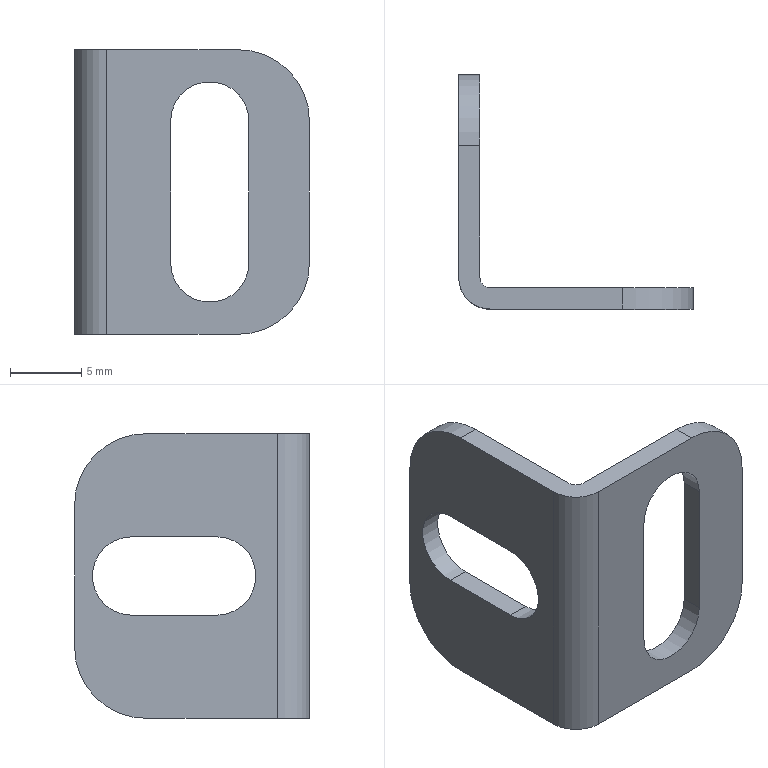Part | NX | features BREP 1 | 1 solid | 22 faces | box 16.5 x 16.5 x 20 mm | volume 690.393 mm3 | plane 12 | cylinder 10 | commonest cylinder face diameters 5.5 x4 10 x4 1.473 x1 4.473 x1
STEP:
#1=CARTESIAN_POINT('',(5.25,-1.5,5.));
#2=VERTEX_POINT('',#1);
#3=CARTESIAN_POINT('',(10.75,-1.5,5.));
#4=VERTEX_POINT('',#3);
#5=CARTESIAN_POINT('',(8.,-1.5,5.));
#6=DIRECTION('',(0.,1.,0.));
#7=DIRECTION('',(0.,0.,1.));
#8=AXIS2_PLACEMENT_3D('',#5,#6,#7);
#9=CIRCLE('',#8,2.75);
#10=EDGE_CURVE('',#2,#4,#9,.T.);
#11=ORIENTED_EDGE('',*,*,#10,.F.);
#12=CARTESIAN_POINT('',(5.25,0.,5.));
#13=VERTEX_POINT('',#12);
#14=CARTESIAN_POINT('',(5.25,-10.,5.));
#15=DIRECTION('',(0.,1.,0.));
#16=VECTOR('',#15,1000.);
#17=LINE('',#14,#16);
#18=EDGE_CURVE('',#2,#13,#17,.T.);
#19=ORIENTED_EDGE('',*,*,#18,.T.);
#20=CARTESIAN_POINT('',(10.75,0.,5.));
#21=VERTEX_POINT('',#20);
#22=CARTESIAN_POINT('',(8.,0.,5.));
#23=DIRECTION('',(0.,1.,0.));
#24=DIRECTION('',(0.,0.,1.));
#25=AXIS2_PLACEMENT_3D('',#22,#23,#24);
#26=CIRCLE('',#25,2.75);
#27=EDGE_CURVE('',#13,#21,#26,.T.);
#28=ORIENTED_EDGE('',*,*,#27,.T.);
#29=CARTESIAN_POINT('',(10.75,-10.,5.));
#30=DIRECTION('',(0.,1.,0.));
#31=VECTOR('',#30,1000.);
#32=LINE('',#29,#31);
#33=EDGE_CURVE('',#4,#21,#32,.T.);
#34=ORIENTED_EDGE('',*,*,#33,.F.);
#35=EDGE_LOOP('',(#11,#19,#28,#34));
#36=FACE_BOUND('',#35,.T.);
#37=CARTESIAN_POINT('',(8.,-10.,5.));
#38=DIRECTION('',(0.,1.,0.));
#39=DIRECTION('',(0.,0.,1.));
#40=AXIS2_PLACEMENT_3D('',#37,#38,#39);
#41=CYLINDRICAL_SURFACE('',#40,2.75);
#42=ADVANCED_FACE('',(#36),#41,.F.);
#43=CARTESIAN_POINT('',(-1.5,11.,-2.75));
#44=VERTEX_POINT('',#43);
#45=CARTESIAN_POINT('',(-1.5,11.,2.75));
#46=VERTEX_POINT('',#45);
#47=CARTESIAN_POINT('',(-1.5,11.,0.));
#48=DIRECTION('',(1.,0.,0.));
#49=DIRECTION('',(0.,1.,0.));
#50=AXIS2_PLACEMENT_3D('',#47,#48,#49);
#51=CIRCLE('',#50,2.75);
#52=EDGE_CURVE('',#44,#46,#51,.T.);
#53=ORIENTED_EDGE('',*,*,#52,.F.);
#54=CARTESIAN_POINT('',(0.,11.,-2.75));
#55=VERTEX_POINT('',#54);
#56=CARTESIAN_POINT('',(-10.,11.,-2.75));
#57=DIRECTION('',(1.,0.,0.));
#58=VECTOR('',#57,1000.);
#59=LINE('',#56,#58);
#60=EDGE_CURVE('',#44,#55,#59,.T.);
#61=ORIENTED_EDGE('',*,*,#60,.T.);
#62=CARTESIAN_POINT('',(0.,11.,2.75));
#63=VERTEX_POINT('',#62);
#64=CARTESIAN_POINT('',(0.,11.,0.));
#65=DIRECTION('',(1.,0.,0.));
#66=DIRECTION('',(0.,1.,0.));
#67=AXIS2_PLACEMENT_3D('',#64,#65,#66);
#68=CIRCLE('',#67,2.75);
#69=EDGE_CURVE('',#55,#63,#68,.T.);
#70=ORIENTED_EDGE('',*,*,#69,.T.);
#71=CARTESIAN_POINT('',(-10.,11.,2.75));
#72=DIRECTION('',(1.,0.,0.));
#73=VECTOR('',#72,1000.);
#74=LINE('',#71,#73);
#75=EDGE_CURVE('',#46,#63,#74,.T.);
#76=ORIENTED_EDGE('',*,*,#75,.F.);
#77=EDGE_LOOP('',(#53,#61,#70,#76));
#78=FACE_BOUND('',#77,.T.);
#79=CARTESIAN_POINT('',(-10.,11.,0.));
#80=DIRECTION('',(1.,0.,0.));
#81=DIRECTION('',(0.,1.,0.));
#82=AXIS2_PLACEMENT_3D('',#79,#80,#81);
#83=CYLINDRICAL_SURFACE('',#82,2.75);
#84=ADVANCED_FACE('',(#78),#83,.F.);
#85=CARTESIAN_POINT('',(-1.5,0.7366,10.));
#86=VERTEX_POINT('',#85);
#87=CARTESIAN_POINT('',(0.7366,-1.5,10.));
#88=VERTEX_POINT('',#87);
#89=CARTESIAN_POINT('',(0.7366,0.7366,10.));
#90=DIRECTION('',(0.,0.,1.));
#91=DIRECTION('',(1.,0.,0.));
#92=AXIS2_PLACEMENT_3D('',#89,#90,#91);
#93=CIRCLE('',#92,2.237);
#94=EDGE_CURVE('',#86,#88,#93,.T.);
#95=ORIENTED_EDGE('',*,*,#94,.T.);
#96=CARTESIAN_POINT('',(10.,-1.5,10.));
#97=VERTEX_POINT('',#96);
#98=CARTESIAN_POINT('',(0.,-1.5,10.));
#99=DIRECTION('',(1.,0.,0.));
#100=VECTOR('',#99,1000.);
#101=LINE('',#98,#100);
#102=EDGE_CURVE('',#88,#97,#101,.T.);
#103=ORIENTED_EDGE('',*,*,#102,.T.);
#104=CARTESIAN_POINT('',(10.,0.,10.));
#105=VERTEX_POINT('',#104);
#106=CARTESIAN_POINT('',(10.,0.7366,10.));
#107=DIRECTION('',(0.,1.,0.));
#108=VECTOR('',#107,1000.);
#109=LINE('',#106,#108);
#110=EDGE_CURVE('',#97,#105,#109,.T.);
#111=ORIENTED_EDGE('',*,*,#110,.T.);
#112=CARTESIAN_POINT('',(0.7366,0.,10.));
#113=VERTEX_POINT('',#112);
#114=CARTESIAN_POINT('',(0.,0.,10.));
#115=DIRECTION('',(1.,0.,0.));
#116=VECTOR('',#115,1000.);
#117=LINE('',#114,#116);
#118=EDGE_CURVE('',#113,#105,#117,.T.);
#119=ORIENTED_EDGE('',*,*,#118,.F.);
#120=CARTESIAN_POINT('',(0.,0.7366,10.));
#121=VERTEX_POINT('',#120);
#122=CARTESIAN_POINT('',(0.7366,0.7366,10.));
#123=DIRECTION('',(0.,0.,1.));
#124=DIRECTION('',(-1.,0.,0.));
#125=AXIS2_PLACEMENT_3D('',#122,#123,#124);
#126=CIRCLE('',#125,0.7366);
#127=EDGE_CURVE('',#121,#113,#126,.T.);
#128=ORIENTED_EDGE('',*,*,#127,.F.);
#129=CARTESIAN_POINT('',(0.,10.,10.));
#130=VERTEX_POINT('',#129);
#131=CARTESIAN_POINT('',(0.,15.,10.));
#132=DIRECTION('',(0.,-1.,0.));
#133=VECTOR('',#132,1000.);
#134=LINE('',#131,#133);
#135=EDGE_CURVE('',#130,#121,#134,.T.);
#136=ORIENTED_EDGE('',*,*,#135,.F.);
#137=CARTESIAN_POINT('',(-1.5,10.,10.));
#138=VERTEX_POINT('',#137);
#139=CARTESIAN_POINT('',(-1.5,10.,10.));
#140=DIRECTION('',(-1.,0.,0.));
#141=VECTOR('',#140,1000.);
#142=LINE('',#139,#141);
#143=EDGE_CURVE('',#130,#138,#142,.T.);
#144=ORIENTED_EDGE('',*,*,#143,.T.);
#145=CARTESIAN_POINT('',(-1.5,15.,10.));
#146=DIRECTION('',(0.,-1.,0.));
#147=VECTOR('',#146,1000.);
#148=LINE('',#145,#147);
#149=EDGE_CURVE('',#138,#86,#148,.T.);
#150=ORIENTED_EDGE('',*,*,#149,.T.);
#151=EDGE_LOOP('',(#95,#103,#111,#119,#128,#136,#144,#150));
#152=FACE_BOUND('',#151,.T.);
#153=CARTESIAN_POINT('',(0.7366,0.,10.));
#154=DIRECTION('',(0.,0.,1.));
#155=DIRECTION('',(1.,0.,0.));
#156=AXIS2_PLACEMENT_3D('',#153,#154,#155);
#157=PLANE('',#156);
#158=ADVANCED_FACE('',(#152),#157,.T.);
#159=CARTESIAN_POINT('',(-1.5,0.7366,-10.));
#160=VERTEX_POINT('',#159);
#161=CARTESIAN_POINT('',(0.7366,-1.5,-10.));
#162=VERTEX_POINT('',#161);
#163=CARTESIAN_POINT('',(0.7366,0.7366,-10.));
#164=DIRECTION('',(0.,0.,1.));
#165=DIRECTION('',(1.,0.,0.));
#166=AXIS2_PLACEMENT_3D('',#163,#164,#165);
#167=CIRCLE('',#166,2.237);
#168=EDGE_CURVE('',#160,#162,#167,.T.);
#169=ORIENTED_EDGE('',*,*,#168,.F.);
#170=CARTESIAN_POINT('',(-1.5,10.,-10.));
#171=VERTEX_POINT('',#170);
#172=CARTESIAN_POINT('',(-1.5,15.,-10.));
#173=DIRECTION('',(0.,-1.,0.));
#174=VECTOR('',#173,1000.);
#175=LINE('',#172,#174);
#176=EDGE_CURVE('',#171,#160,#175,.T.);
#177=ORIENTED_EDGE('',*,*,#176,.F.);
#178=CARTESIAN_POINT('',(0.,10.,-10.));
#179=VERTEX_POINT('',#178);
#180=CARTESIAN_POINT('',(0.7366,10.,-10.));
#181=DIRECTION('',(1.,0.,0.));
#182=VECTOR('',#181,1000.);
#183=LINE('',#180,#182);
#184=EDGE_CURVE('',#171,#179,#183,.T.);
#185=ORIENTED_EDGE('',*,*,#184,.T.);
#186=CARTESIAN_POINT('',(0.,0.7366,-10.));
#187=VERTEX_POINT('',#186);
#188=CARTESIAN_POINT('',(0.,15.,-10.));
#189=DIRECTION('',(0.,-1.,0.));
#190=VECTOR('',#189,1000.);
#191=LINE('',#188,#190);
#192=EDGE_CURVE('',#179,#187,#191,.T.);
#193=ORIENTED_EDGE('',*,*,#192,.T.);
#194=CARTESIAN_POINT('',(0.7366,0.,-10.));
#195=VERTEX_POINT('',#194);
#196=CARTESIAN_POINT('',(0.7366,0.7366,-10.));
#197=DIRECTION('',(0.,0.,1.));
#198=DIRECTION('',(-1.,0.,0.));
#199=AXIS2_PLACEMENT_3D('',#196,#197,#198);
#200=CIRCLE('',#199,0.7366);
#201=EDGE_CURVE('',#187,#195,#200,.T.);
#202=ORIENTED_EDGE('',*,*,#201,.T.);
#203=CARTESIAN_POINT('',(10.,0.,-10.));
#204=VERTEX_POINT('',#203);
#205=CARTESIAN_POINT('',(0.,0.,-10.));
#206=DIRECTION('',(1.,0.,0.));
#207=VECTOR('',#206,1000.);
#208=LINE('',#205,#207);
#209=EDGE_CURVE('',#195,#204,#208,.T.);
#210=ORIENTED_EDGE('',*,*,#209,.T.);
#211=CARTESIAN_POINT('',(10.,-1.5,-10.));
#212=VERTEX_POINT('',#211);
#213=CARTESIAN_POINT('',(10.,0.7366,-10.));
#214=DIRECTION('',(0.,-1.,0.));
#215=VECTOR('',#214,1000.);
#216=LINE('',#213,#215);
#217=EDGE_CURVE('',#204,#212,#216,.T.);
#218=ORIENTED_EDGE('',*,*,#217,.T.);
#219=CARTESIAN_POINT('',(0.,-1.5,-10.));
#220=DIRECTION('',(1.,0.,0.));
#221=VECTOR('',#220,1000.);
#222=LINE('',#219,#221);
#223=EDGE_CURVE('',#162,#212,#222,.T.);
#224=ORIENTED_EDGE('',*,*,#223,.F.);
#225=EDGE_LOOP('',(#169,#177,#185,#193,#202,#210,#218,#224));
#226=FACE_BOUND('',#225,.T.);
#227=CARTESIAN_POINT('',(0.,0.7366,-10.));
#228=DIRECTION('',(0.,0.,-1.));
#229=DIRECTION('',(-1.,0.,0.));
#230=AXIS2_PLACEMENT_3D('',#227,#228,#229);
#231=PLANE('',#230);
#232=ADVANCED_FACE('',(#226),#231,.T.);
#233=CARTESIAN_POINT('',(10.75,-1.5,-5.));
#234=VERTEX_POINT('',#233);
#235=CARTESIAN_POINT('',(10.75,-1.5,10.));
#236=DIRECTION('',(0.,0.,-1.));
#237=VECTOR('',#236,1000.);
#238=LINE('',#235,#237);
#239=EDGE_CURVE('',#4,#234,#238,.T.);
#240=ORIENTED_EDGE('',*,*,#239,.T.);
#241=CARTESIAN_POINT('',(5.25,-1.5,-5.));
#242=VERTEX_POINT('',#241);
#243=CARTESIAN_POINT('',(8.,-1.5,-5.));
#244=DIRECTION('',(0.,1.,0.));
#245=DIRECTION('',(0.,0.,1.));
#246=AXIS2_PLACEMENT_3D('',#243,#244,#245);
#247=CIRCLE('',#246,2.75);
#248=EDGE_CURVE('',#234,#242,#247,.T.);
#249=ORIENTED_EDGE('',*,*,#248,.T.);
#250=CARTESIAN_POINT('',(5.25,-1.5,10.));
#251=DIRECTION('',(0.,0.,1.));
#252=VECTOR('',#251,1000.);
#253=LINE('',#250,#252);
#254=EDGE_CURVE('',#242,#2,#253,.T.);
#255=ORIENTED_EDGE('',*,*,#254,.T.);
#256=ORIENTED_EDGE('',*,*,#10,.T.);
#257=EDGE_LOOP('',(#240,#249,#255,#256));
#258=FACE_BOUND('',#257,.T.);
#259=ORIENTED_EDGE('',*,*,#223,.T.);
#260=CARTESIAN_POINT('',(15.,-1.5,-5.));
#261=VERTEX_POINT('',#260);
#262=CARTESIAN_POINT('',(10.,-1.5,-5.));
#263=DIRECTION('',(0.,-1.,0.));
#264=DIRECTION('',(0.,0.,1.));
#265=AXIS2_PLACEMENT_3D('',#262,#263,#264);
#266=CIRCLE('',#265,5.);
#267=EDGE_CURVE('',#212,#261,#266,.T.);
#268=ORIENTED_EDGE('',*,*,#267,.T.);
#269=CARTESIAN_POINT('',(15.,-1.5,5.));
#270=VERTEX_POINT('',#269);
#271=CARTESIAN_POINT('',(15.,-1.5,10.));
#272=DIRECTION('',(0.,0.,-1.));
#273=VECTOR('',#272,1000.);
#274=LINE('',#271,#273);
#275=EDGE_CURVE('',#270,#261,#274,.T.);
#276=ORIENTED_EDGE('',*,*,#275,.F.);
#277=CARTESIAN_POINT('',(10.,-1.5,5.));
#278=DIRECTION('',(0.,-1.,0.));
#279=DIRECTION('',(0.,0.,1.));
#280=AXIS2_PLACEMENT_3D('',#277,#278,#279);
#281=CIRCLE('',#280,5.);
#282=EDGE_CURVE('',#270,#97,#281,.T.);
#283=ORIENTED_EDGE('',*,*,#282,.T.);
#284=ORIENTED_EDGE('',*,*,#102,.F.);
#285=CARTESIAN_POINT('',(0.7366,-1.5,10.));
#286=DIRECTION('',(0.,0.,-1.));
#287=VECTOR('',#286,1000.);
#288=LINE('',#285,#287);
#289=EDGE_CURVE('',#88,#162,#288,.T.);
#290=ORIENTED_EDGE('',*,*,#289,.T.);
#291=EDGE_LOOP('',(#259,#268,#276,#283,#284,#290));
#292=FACE_BOUND('',#291,.T.);
#293=CARTESIAN_POINT('',(0.,-1.5,10.));
#294=DIRECTION('',(0.,1.,0.));
#295=DIRECTION('',(0.,0.,1.));
#296=AXIS2_PLACEMENT_3D('',#293,#294,#295);
#297=PLANE('',#296);
#298=ADVANCED_FACE('',(#258,#292),#297,.F.);
#299=ORIENTED_EDGE('',*,*,#275,.T.);
#300=CARTESIAN_POINT('',(15.,0.,-5.));
#301=VERTEX_POINT('',#300);
#302=CARTESIAN_POINT('',(15.,0.,-5.));
#303=DIRECTION('',(0.,1.,0.));
#304=VECTOR('',#303,1000.);
#305=LINE('',#302,#304);
#306=EDGE_CURVE('',#261,#301,#305,.T.);
#307=ORIENTED_EDGE('',*,*,#306,.T.);
#308=CARTESIAN_POINT('',(15.,0.,5.));
#309=VERTEX_POINT('',#308);
#310=CARTESIAN_POINT('',(15.,0.,10.));
#311=DIRECTION('',(0.,0.,-1.));
#312=VECTOR('',#311,1000.);
#313=LINE('',#310,#312);
#314=EDGE_CURVE('',#309,#301,#313,.T.);
#315=ORIENTED_EDGE('',*,*,#314,.F.);
#316=CARTESIAN_POINT('',(15.,0.,5.));
#317=DIRECTION('',(0.,-1.,0.));
#318=VECTOR('',#317,1000.);
#319=LINE('',#316,#318);
#320=EDGE_CURVE('',#309,#270,#319,.T.);
#321=ORIENTED_EDGE('',*,*,#320,.T.);
#322=EDGE_LOOP('',(#299,#307,#315,#321));
#323=FACE_BOUND('',#322,.T.);
#324=CARTESIAN_POINT('',(15.,0.,10.));
#325=DIRECTION('',(1.,0.,0.));
#326=DIRECTION('',(0.,0.,-1.));
#327=AXIS2_PLACEMENT_3D('',#324,#325,#326);
#328=PLANE('',#327);
#329=ADVANCED_FACE('',(#323),#328,.T.);
#330=CARTESIAN_POINT('',(10.75,0.,-5.));
#331=VERTEX_POINT('',#330);
#332=CARTESIAN_POINT('',(5.25,0.,-5.));
#333=VERTEX_POINT('',#332);
#334=CARTESIAN_POINT('',(8.,0.,-5.));
#335=DIRECTION('',(0.,1.,0.));
#336=DIRECTION('',(0.,0.,1.));
#337=AXIS2_PLACEMENT_3D('',#334,#335,#336);
#338=CIRCLE('',#337,2.75);
#339=EDGE_CURVE('',#331,#333,#338,.T.);
#340=ORIENTED_EDGE('',*,*,#339,.F.);
#341=CARTESIAN_POINT('',(10.75,0.,-5.));
#342=DIRECTION('',(0.,0.,-1.));
#343=VECTOR('',#342,1000.);
#344=LINE('',#341,#343);
#345=EDGE_CURVE('',#21,#331,#344,.T.);
#346=ORIENTED_EDGE('',*,*,#345,.F.);
#347=ORIENTED_EDGE('',*,*,#27,.F.);
#348=CARTESIAN_POINT('',(5.25,0.,-5.));
#349=DIRECTION('',(0.,0.,1.));
#350=VECTOR('',#349,1000.);
#351=LINE('',#348,#350);
#352=EDGE_CURVE('',#333,#13,#351,.T.);
#353=ORIENTED_EDGE('',*,*,#352,.F.);
#354=EDGE_LOOP('',(#340,#346,#347,#353));
#355=FACE_BOUND('',#354,.T.);
#356=ORIENTED_EDGE('',*,*,#314,.T.);
#357=CARTESIAN_POINT('',(10.,0.,-5.));
#358=DIRECTION('',(0.,1.,0.));
#359=DIRECTION('',(0.,0.,1.));
#360=AXIS2_PLACEMENT_3D('',#357,#358,#359);
#361=CIRCLE('',#360,5.);
#362=EDGE_CURVE('',#301,#204,#361,.T.);
#363=ORIENTED_EDGE('',*,*,#362,.T.);
#364=ORIENTED_EDGE('',*,*,#209,.F.);
#365=CARTESIAN_POINT('',(0.7366,0.,10.));
#366=DIRECTION('',(0.,0.,-1.));
#367=VECTOR('',#366,1000.);
#368=LINE('',#365,#367);
#369=EDGE_CURVE('',#113,#195,#368,.T.);
#370=ORIENTED_EDGE('',*,*,#369,.F.);
#371=ORIENTED_EDGE('',*,*,#118,.T.);
#372=CARTESIAN_POINT('',(10.,0.,5.));
#373=DIRECTION('',(0.,1.,0.));
#374=DIRECTION('',(0.,0.,1.));
#375=AXIS2_PLACEMENT_3D('',#372,#373,#374);
#376=CIRCLE('',#375,5.);
#377=EDGE_CURVE('',#105,#309,#376,.T.);
#378=ORIENTED_EDGE('',*,*,#377,.T.);
#379=EDGE_LOOP('',(#356,#363,#364,#370,#371,#378));
#380=FACE_BOUND('',#379,.T.);
#381=CARTESIAN_POINT('',(0.,0.,10.));
#382=DIRECTION('',(0.,1.,0.));
#383=DIRECTION('',(0.,0.,1.));
#384=AXIS2_PLACEMENT_3D('',#381,#382,#383);
#385=PLANE('',#384);
#386=ADVANCED_FACE('',(#355,#380),#385,.T.);
#387=ORIENTED_EDGE('',*,*,#201,.F.);
#388=CARTESIAN_POINT('',(0.,0.7366,10.));
#389=DIRECTION('',(0.,0.,-1.));
#390=VECTOR('',#389,1000.);
#391=LINE('',#388,#390);
#392=EDGE_CURVE('',#121,#187,#391,.T.);
#393=ORIENTED_EDGE('',*,*,#392,.F.);
#394=ORIENTED_EDGE('',*,*,#127,.T.);
#395=ORIENTED_EDGE('',*,*,#369,.T.);
#396=EDGE_LOOP('',(#387,#393,#394,#395));
#397=FACE_BOUND('',#396,.T.);
#398=CARTESIAN_POINT('',(0.7366,0.7366,10.));
#399=DIRECTION('',(0.,0.,-1.));
#400=DIRECTION('',(-1.,0.,0.));
#401=AXIS2_PLACEMENT_3D('',#398,#399,#400);
#402=CYLINDRICAL_SURFACE('',#401,0.7366);
#403=ADVANCED_FACE('',(#397),#402,.F.);
#404=ORIENTED_EDGE('',*,*,#69,.F.);
#405=CARTESIAN_POINT('',(0.,5.,-2.75));
#406=VERTEX_POINT('',#405);
#407=CARTESIAN_POINT('',(0.,11.,-2.75));
#408=DIRECTION('',(0.,1.,0.));
#409=VECTOR('',#408,1000.);
#410=LINE('',#407,#409);
#411=EDGE_CURVE('',#406,#55,#410,.T.);
#412=ORIENTED_EDGE('',*,*,#411,.F.);
#413=CARTESIAN_POINT('',(0.,5.,2.75));
#414=VERTEX_POINT('',#413);
#415=CARTESIAN_POINT('',(0.,5.,0.));
#416=DIRECTION('',(1.,0.,0.));
#417=DIRECTION('',(0.,1.,0.));
#418=AXIS2_PLACEMENT_3D('',#415,#416,#417);
#419=CIRCLE('',#418,2.75);
#420=EDGE_CURVE('',#414,#406,#419,.T.);
#421=ORIENTED_EDGE('',*,*,#420,.F.);
#422=CARTESIAN_POINT('',(0.,11.,2.75));
#423=DIRECTION('',(0.,-1.,0.));
#424=VECTOR('',#423,1000.);
#425=LINE('',#422,#424);
#426=EDGE_CURVE('',#63,#414,#425,.T.);
#427=ORIENTED_EDGE('',*,*,#426,.F.);
#428=EDGE_LOOP('',(#404,#412,#421,#427));
#429=FACE_BOUND('',#428,.T.);
#430=CARTESIAN_POINT('',(0.,15.,5.));
#431=VERTEX_POINT('',#430);
#432=CARTESIAN_POINT('',(0.,15.,-5.));
#433=VERTEX_POINT('',#432);
#434=CARTESIAN_POINT('',(0.,15.,10.));
#435=DIRECTION('',(0.,0.,-1.));
#436=VECTOR('',#435,1000.);
#437=LINE('',#434,#436);
#438=EDGE_CURVE('',#431,#433,#437,.T.);
#439=ORIENTED_EDGE('',*,*,#438,.F.);
#440=CARTESIAN_POINT('',(0.,10.,5.));
#441=DIRECTION('',(1.,0.,0.));
#442=DIRECTION('',(0.,1.,0.));
#443=AXIS2_PLACEMENT_3D('',#440,#441,#442);
#444=CIRCLE('',#443,5.);
#445=EDGE_CURVE('',#431,#130,#444,.T.);
#446=ORIENTED_EDGE('',*,*,#445,.T.);
#447=ORIENTED_EDGE('',*,*,#135,.T.);
#448=ORIENTED_EDGE('',*,*,#392,.T.);
#449=ORIENTED_EDGE('',*,*,#192,.F.);
#450=CARTESIAN_POINT('',(0.,10.,-5.));
#451=DIRECTION('',(1.,0.,0.));
#452=DIRECTION('',(0.,1.,0.));
#453=AXIS2_PLACEMENT_3D('',#450,#451,#452);
#454=CIRCLE('',#453,5.);
#455=EDGE_CURVE('',#179,#433,#454,.T.);
#456=ORIENTED_EDGE('',*,*,#455,.T.);
#457=EDGE_LOOP('',(#439,#446,#447,#448,#449,#456));
#458=FACE_BOUND('',#457,.T.);
#459=CARTESIAN_POINT('',(0.,15.,10.));
#460=DIRECTION('',(1.,0.,0.));
#461=DIRECTION('',(0.,1.,0.));
#462=AXIS2_PLACEMENT_3D('',#459,#460,#461);
#463=PLANE('',#462);
#464=ADVANCED_FACE('',(#429,#458),#463,.T.);
#465=CARTESIAN_POINT('',(-1.5,15.,5.));
#466=VERTEX_POINT('',#465);
#467=CARTESIAN_POINT('',(-1.5,15.,-5.));
#468=VERTEX_POINT('',#467);
#469=CARTESIAN_POINT('',(-1.5,15.,10.));
#470=DIRECTION('',(0.,0.,-1.));
#471=VECTOR('',#470,1000.);
#472=LINE('',#469,#471);
#473=EDGE_CURVE('',#466,#468,#472,.T.);
#474=ORIENTED_EDGE('',*,*,#473,.F.);
#475=CARTESIAN_POINT('',(0.,15.,5.));
#476=DIRECTION('',(1.,0.,0.));
#477=VECTOR('',#476,1000.);
#478=LINE('',#475,#477);
#479=EDGE_CURVE('',#466,#431,#478,.T.);
#480=ORIENTED_EDGE('',*,*,#479,.T.);
#481=ORIENTED_EDGE('',*,*,#438,.T.);
#482=CARTESIAN_POINT('',(-1.5,15.,-5.));
#483=DIRECTION('',(-1.,0.,0.));
#484=VECTOR('',#483,1000.);
#485=LINE('',#482,#484);
#486=EDGE_CURVE('',#433,#468,#485,.T.);
#487=ORIENTED_EDGE('',*,*,#486,.T.);
#488=EDGE_LOOP('',(#474,#480,#481,#487));
#489=FACE_BOUND('',#488,.T.);
#490=CARTESIAN_POINT('',(-1.5,15.,10.));
#491=DIRECTION('',(0.,1.,0.));
#492=DIRECTION('',(0.,0.,1.));
#493=AXIS2_PLACEMENT_3D('',#490,#491,#492);
#494=PLANE('',#493);
#495=ADVANCED_FACE('',(#489),#494,.T.);
#496=CARTESIAN_POINT('',(-1.5,5.,-2.75));
#497=VERTEX_POINT('',#496);
#498=CARTESIAN_POINT('',(-1.5,15.,-2.75));
#499=DIRECTION('',(0.,1.,0.));
#500=VECTOR('',#499,1000.);
#501=LINE('',#498,#500);
#502=EDGE_CURVE('',#497,#44,#501,.T.);
#503=ORIENTED_EDGE('',*,*,#502,.T.);
#504=ORIENTED_EDGE('',*,*,#52,.T.);
#505=CARTESIAN_POINT('',(-1.5,5.,2.75));
#506=VERTEX_POINT('',#505);
#507=CARTESIAN_POINT('',(-1.5,15.,2.75));
#508=DIRECTION('',(0.,-1.,0.));
#509=VECTOR('',#508,1000.);
#510=LINE('',#507,#509);
#511=EDGE_CURVE('',#46,#506,#510,.T.);
#512=ORIENTED_EDGE('',*,*,#511,.T.);
#513=CARTESIAN_POINT('',(-1.5,5.,0.));
#514=DIRECTION('',(1.,0.,0.));
#515=DIRECTION('',(0.,1.,0.));
#516=AXIS2_PLACEMENT_3D('',#513,#514,#515);
#517=CIRCLE('',#516,2.75);
#518=EDGE_CURVE('',#506,#497,#517,.T.);
#519=ORIENTED_EDGE('',*,*,#518,.T.);
#520=EDGE_LOOP('',(#503,#504,#512,#519));
#521=FACE_BOUND('',#520,.T.);
#522=ORIENTED_EDGE('',*,*,#149,.F.);
#523=CARTESIAN_POINT('',(-1.5,10.,5.));
#524=DIRECTION('',(-1.,0.,0.));
#525=DIRECTION('',(0.,1.,0.));
#526=AXIS2_PLACEMENT_3D('',#523,#524,#525);
#527=CIRCLE('',#526,5.);
#528=EDGE_CURVE('',#138,#466,#527,.T.);
#529=ORIENTED_EDGE('',*,*,#528,.T.);
#530=ORIENTED_EDGE('',*,*,#473,.T.);
#531=CARTESIAN_POINT('',(-1.5,10.,-5.));
#532=DIRECTION('',(-1.,0.,0.));
#533=DIRECTION('',(0.,1.,0.));
#534=AXIS2_PLACEMENT_3D('',#531,#532,#533);
#535=CIRCLE('',#534,5.);
#536=EDGE_CURVE('',#468,#171,#535,.T.);
#537=ORIENTED_EDGE('',*,*,#536,.T.);
#538=ORIENTED_EDGE('',*,*,#176,.T.);
#539=CARTESIAN_POINT('',(-1.5,0.7366,10.));
#540=DIRECTION('',(0.,0.,-1.));
#541=VECTOR('',#540,1000.);
#542=LINE('',#539,#541);
#543=EDGE_CURVE('',#86,#160,#542,.T.);
#544=ORIENTED_EDGE('',*,*,#543,.F.);
#545=EDGE_LOOP('',(#522,#529,#530,#537,#538,#544));
#546=FACE_BOUND('',#545,.T.);
#547=CARTESIAN_POINT('',(-1.5,15.,10.));
#548=DIRECTION('',(1.,0.,0.));
#549=DIRECTION('',(0.,1.,0.));
#550=AXIS2_PLACEMENT_3D('',#547,#548,#549);
#551=PLANE('',#550);
#552=ADVANCED_FACE('',(#521,#546),#551,.F.);
#553=ORIENTED_EDGE('',*,*,#168,.T.);
#554=ORIENTED_EDGE('',*,*,#289,.F.);
#555=ORIENTED_EDGE('',*,*,#94,.F.);
#556=ORIENTED_EDGE('',*,*,#543,.T.);
#557=EDGE_LOOP('',(#553,#554,#555,#556));
#558=FACE_BOUND('',#557,.T.);
#559=CARTESIAN_POINT('',(0.7366,0.7366,10.));
#560=DIRECTION('',(0.,0.,-1.));
#561=DIRECTION('',(-1.,0.,0.));
#562=AXIS2_PLACEMENT_3D('',#559,#560,#561);
#563=CYLINDRICAL_SURFACE('',#562,2.237);
#564=ADVANCED_FACE('',(#558),#563,.T.);
#565=ORIENTED_EDGE('',*,*,#362,.F.);
#566=ORIENTED_EDGE('',*,*,#306,.F.);
#567=ORIENTED_EDGE('',*,*,#267,.F.);
#568=ORIENTED_EDGE('',*,*,#217,.F.);
#569=EDGE_LOOP('',(#565,#566,#567,#568));
#570=FACE_BOUND('',#569,.T.);
#571=CARTESIAN_POINT('',(10.,0.7366,-5.));
#572=DIRECTION('',(0.,-1.,0.));
#573=DIRECTION('',(0.,0.,-1.));
#574=AXIS2_PLACEMENT_3D('',#571,#572,#573);
#575=CYLINDRICAL_SURFACE('',#574,5.);
#576=ADVANCED_FACE('',(#570),#575,.T.);
#577=ORIENTED_EDGE('',*,*,#377,.F.);
#578=ORIENTED_EDGE('',*,*,#110,.F.);
#579=ORIENTED_EDGE('',*,*,#282,.F.);
#580=ORIENTED_EDGE('',*,*,#320,.F.);
#581=EDGE_LOOP('',(#577,#578,#579,#580));
#582=FACE_BOUND('',#581,.T.);
#583=CARTESIAN_POINT('',(10.,0.,5.));
#584=DIRECTION('',(0.,-1.,0.));
#585=DIRECTION('',(0.,0.,-1.));
#586=AXIS2_PLACEMENT_3D('',#583,#584,#585);
#587=CYLINDRICAL_SURFACE('',#586,5.);
#588=ADVANCED_FACE('',(#582),#587,.T.);
#589=ORIENTED_EDGE('',*,*,#528,.F.);
#590=ORIENTED_EDGE('',*,*,#143,.F.);
#591=ORIENTED_EDGE('',*,*,#445,.F.);
#592=ORIENTED_EDGE('',*,*,#479,.F.);
#593=EDGE_LOOP('',(#589,#590,#591,#592));
#594=FACE_BOUND('',#593,.T.);
#595=CARTESIAN_POINT('',(-1.5,10.,5.));
#596=DIRECTION('',(-1.,0.,0.));
#597=DIRECTION('',(0.,0.,1.));
#598=AXIS2_PLACEMENT_3D('',#595,#596,#597);
#599=CYLINDRICAL_SURFACE('',#598,5.);
#600=ADVANCED_FACE('',(#594),#599,.T.);
#601=ORIENTED_EDGE('',*,*,#536,.F.);
#602=ORIENTED_EDGE('',*,*,#486,.F.);
#603=ORIENTED_EDGE('',*,*,#455,.F.);
#604=ORIENTED_EDGE('',*,*,#184,.F.);
#605=EDGE_LOOP('',(#601,#602,#603,#604));
#606=FACE_BOUND('',#605,.T.);
#607=CARTESIAN_POINT('',(0.7366,10.,-5.));
#608=DIRECTION('',(1.,0.,0.));
#609=DIRECTION('',(0.,0.,-1.));
#610=AXIS2_PLACEMENT_3D('',#607,#608,#609);
#611=CYLINDRICAL_SURFACE('',#610,5.);
#612=ADVANCED_FACE('',(#606),#611,.T.);
#613=CARTESIAN_POINT('',(-10.,5.,-2.75));
#614=DIRECTION('',(1.,0.,0.));
#615=VECTOR('',#614,1000.);
#616=LINE('',#613,#615);
#617=EDGE_CURVE('',#497,#406,#616,.T.);
#618=ORIENTED_EDGE('',*,*,#617,.T.);
#619=ORIENTED_EDGE('',*,*,#411,.T.);
#620=ORIENTED_EDGE('',*,*,#60,.F.);
#621=ORIENTED_EDGE('',*,*,#502,.F.);
#622=EDGE_LOOP('',(#618,#619,#620,#621));
#623=FACE_BOUND('',#622,.T.);
#624=CARTESIAN_POINT('',(-10.,11.,-2.75));
#625=DIRECTION('',(0.,0.,-1.));
#626=DIRECTION('',(0.,1.,0.));
#627=AXIS2_PLACEMENT_3D('',#624,#625,#626);
#628=PLANE('',#627);
#629=ADVANCED_FACE('',(#623),#628,.F.);
#630=CARTESIAN_POINT('',(-10.,5.,2.75));
#631=DIRECTION('',(1.,0.,0.));
#632=VECTOR('',#631,1000.);
#633=LINE('',#630,#632);
#634=EDGE_CURVE('',#506,#414,#633,.T.);
#635=ORIENTED_EDGE('',*,*,#634,.T.);
#636=ORIENTED_EDGE('',*,*,#420,.T.);
#637=ORIENTED_EDGE('',*,*,#617,.F.);
#638=ORIENTED_EDGE('',*,*,#518,.F.);
#639=EDGE_LOOP('',(#635,#636,#637,#638));
#640=FACE_BOUND('',#639,.T.);
#641=CARTESIAN_POINT('',(-10.,5.,0.));
#642=DIRECTION('',(1.,0.,0.));
#643=DIRECTION('',(0.,1.,0.));
#644=AXIS2_PLACEMENT_3D('',#641,#642,#643);
#645=CYLINDRICAL_SURFACE('',#644,2.75);
#646=ADVANCED_FACE('',(#640),#645,.F.);
#647=ORIENTED_EDGE('',*,*,#75,.T.);
#648=ORIENTED_EDGE('',*,*,#426,.T.);
#649=ORIENTED_EDGE('',*,*,#634,.F.);
#650=ORIENTED_EDGE('',*,*,#511,.F.);
#651=EDGE_LOOP('',(#647,#648,#649,#650));
#652=FACE_BOUND('',#651,.T.);
#653=CARTESIAN_POINT('',(-10.,11.,2.75));
#654=DIRECTION('',(0.,0.,1.));
#655=DIRECTION('',(0.,-1.,0.));
#656=AXIS2_PLACEMENT_3D('',#653,#654,#655);
#657=PLANE('',#656);
#658=ADVANCED_FACE('',(#652),#657,.F.);
#659=CARTESIAN_POINT('',(10.75,-10.,-5.));
#660=DIRECTION('',(0.,1.,0.));
#661=VECTOR('',#660,1000.);
#662=LINE('',#659,#661);
#663=EDGE_CURVE('',#234,#331,#662,.T.);
#664=ORIENTED_EDGE('',*,*,#663,.T.);
#665=ORIENTED_EDGE('',*,*,#339,.T.);
#666=CARTESIAN_POINT('',(5.25,-10.,-5.));
#667=DIRECTION('',(0.,1.,0.));
#668=VECTOR('',#667,1000.);
#669=LINE('',#666,#668);
#670=EDGE_CURVE('',#242,#333,#669,.T.);
#671=ORIENTED_EDGE('',*,*,#670,.F.);
#672=ORIENTED_EDGE('',*,*,#248,.F.);
#673=EDGE_LOOP('',(#664,#665,#671,#672));
#674=FACE_BOUND('',#673,.T.);
#675=CARTESIAN_POINT('',(8.,-10.,-5.));
#676=DIRECTION('',(0.,1.,0.));
#677=DIRECTION('',(0.,0.,1.));
#678=AXIS2_PLACEMENT_3D('',#675,#676,#677);
#679=CYLINDRICAL_SURFACE('',#678,2.75);
#680=ADVANCED_FACE('',(#674),#679,.F.);
#681=ORIENTED_EDGE('',*,*,#33,.T.);
#682=ORIENTED_EDGE('',*,*,#345,.T.);
#683=ORIENTED_EDGE('',*,*,#663,.F.);
#684=ORIENTED_EDGE('',*,*,#239,.F.);
#685=EDGE_LOOP('',(#681,#682,#683,#684));
#686=FACE_BOUND('',#685,.T.);
#687=CARTESIAN_POINT('',(10.75,-10.,-5.));
#688=DIRECTION('',(1.,0.,0.));
#689=DIRECTION('',(0.,0.,-1.));
#690=AXIS2_PLACEMENT_3D('',#687,#688,#689);
#691=PLANE('',#690);
#692=ADVANCED_FACE('',(#686),#691,.F.);
#693=ORIENTED_EDGE('',*,*,#670,.T.);
#694=ORIENTED_EDGE('',*,*,#352,.T.);
#695=ORIENTED_EDGE('',*,*,#18,.F.);
#696=ORIENTED_EDGE('',*,*,#254,.F.);
#697=EDGE_LOOP('',(#693,#694,#695,#696));
#698=FACE_BOUND('',#697,.T.);
#699=CARTESIAN_POINT('',(5.25,-10.,-5.));
#700=DIRECTION('',(-1.,0.,0.));
#701=DIRECTION('',(0.,0.,1.));
#702=AXIS2_PLACEMENT_3D('',#699,#700,#701);
#703=PLANE('',#702);
#704=ADVANCED_FACE('',(#698),#703,.F.);
#705=CLOSED_SHELL('',(#42,#84,#158,#232,#298,#329,#386,#403,#464,#495,#552,#564,#576,#588,#600,#612,#629,#646,#658,#680,#692,#704));
#706=MANIFOLD_SOLID_BREP('',#705);
#707=(LENGTH_UNIT()NAMED_UNIT(*)SI_UNIT(.MILLI.,.METRE.));
#708=UNCERTAINTY_MEASURE_WITH_UNIT(LENGTH_MEASURE(0.00001),#707,'','');
#709=(NAMED_UNIT(*)PLANE_ANGLE_UNIT()SI_UNIT($,.RADIAN.));
#710=(NAMED_UNIT(*)SI_UNIT($,.STERADIAN.)SOLID_ANGLE_UNIT());
#711=(GEOMETRIC_REPRESENTATION_CONTEXT(3)GLOBAL_UNCERTAINTY_ASSIGNED_CONTEXT((#708))GLOBAL_UNIT_ASSIGNED_CONTEXT((#707,#709,#710))REPRESENTATION_CONTEXT('',''));
#712=ADVANCED_BREP_SHAPE_REPRESENTATION('',(#706),#711);